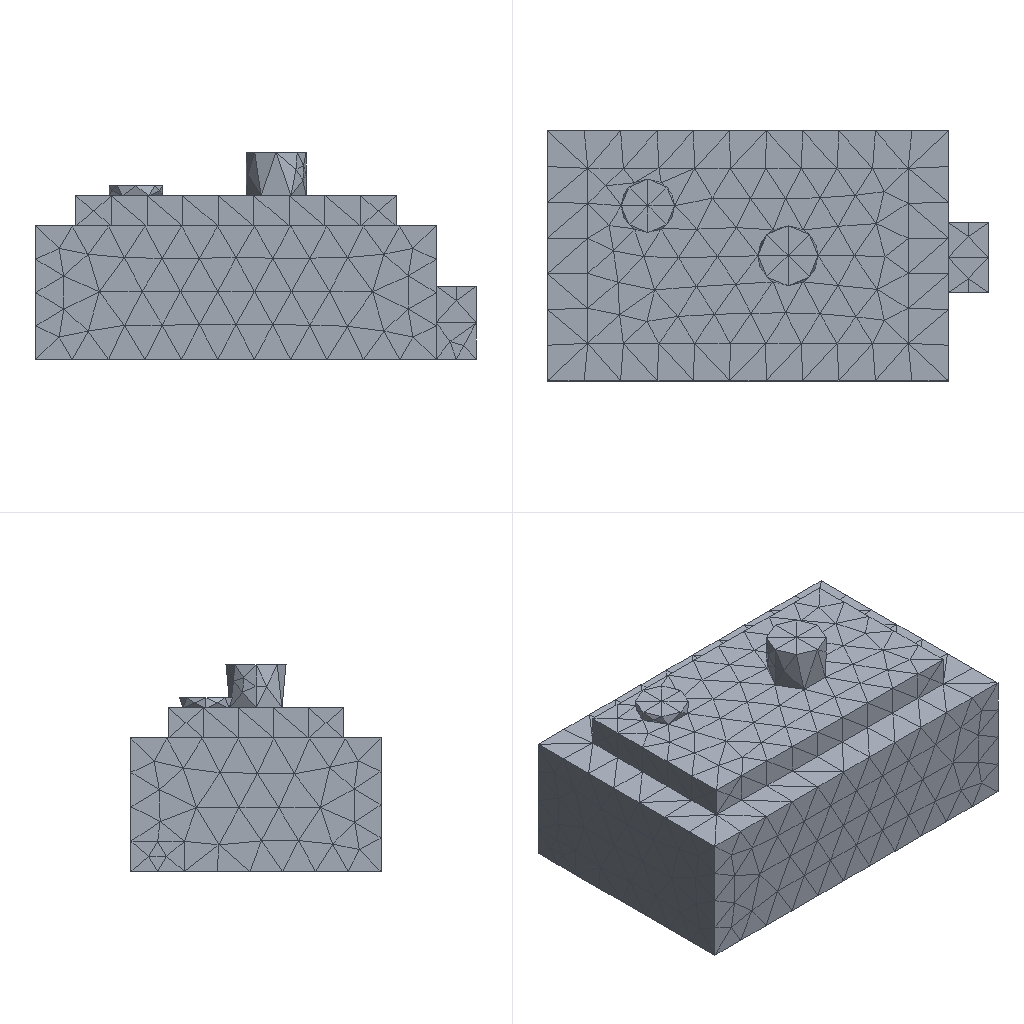Simulation study | ansys mapdl
Set-up summary:
category,name,step,type,value,unit,region
solver,ansys_mapdl
units,mm-N-s-tonne (MPa),,inferred,E=210000 density=
analysis,model,,static
mesh,nodes,,,4843
mesh,elements,,,2901
element_type,SOLID187,,,2901
material,mat 1,,E,210000
material,mat 1,,nu,0.3
load,,model,body load temp,,,all
load,,model,force,"1000 [dir=(0, 0, -1) n=211]",,node list
bc,,model,fixed,"[dofs=UX,UY,UZ n=5226]",,node list
Ansys APDL input file, long lists of numbers shortened:
/COM,ANSYS RELEASE 2026 R1           BUILD 26.1      UP20260202       09:08:46
/PREP7
/NOPR
/TITLE,2
ANTYPE, 0
*IF,_CDRDOFF,EQ,1,THEN     !if solid model was read in
_CDRDOFF=             !reset flag, numoffs already performed
*ELSE              !offset database for the following FE model
NUMOFF,NODE,     4843
NUMOFF,ELEM,     2901
NUMOFF,MAT ,        1
NUMOFF,TYPE,        1
*ENDIF
*SET,_RETURN ,  0.
*SET,_STATUS ,  0.
*SET,_UIQR   ,  211.
*SET,__FLOATPARAMETER__,  4843.
DOF,DELETE
ETBLOCK,        1,        1
(2i9,19a9)
        1      187        0        0        0        0        0        0        0        0        0        0        0        0        0        0        0        0        0        0        0
       -1
NBLOCK,6,SOLID,      4843,      4843
(3i9,6e21.13e3)
        1        0        0-4.4050000000000E+001 3.7500000000000E+001 9.0000000000000E+000
! (4842 more lines like these left out)
N,UNBL,LOC,       -1,
EBLOCK,19,SOLID,      2901,      2901
(19i10)
         1         1         1         1         0         0         0         0        10         0         1      1847      1570      1848      1569      2125      2126      2127      2128
! (5801 more lines like these left out)
        -1
MPTEMP,UNBL, 1, 1,  0.    ,
MPDATA,UNBL, 1,EX  ,       1, 1,  210000.000    ,
MPTEMP,UNBL, 1, 1,  0.    ,
MPDATA,UNBL, 1,NUXY,       1, 1, 0.3    ,
MPTEMP,UNBL, 1, 1,  0.    ,
MPDATA,UNBL, 1,PRXY,       1, 1, 0.3    ,
EXTOPT,ATTR,      0,      0,      0
EXTOPT,ESIZE,  0,  0.
EXTOPT,ACLEAR,      0
TREF,  0.
IRLF,  0
BFUNIF,TEMP,_TINY
ACEL,  0.    ,  0.    ,  0.
OMEGA,  0.    ,  0.    ,  0.
DOMEGA,  0.    ,  0.    ,  0.
CGLOC,  0.    ,  0.    ,  0.
CGOMEGA,  0.    ,  0.    ,  0.
DCGOMG,  0.    ,  0.    ,  0.
KUSE,     0
TIME,  0.
ALPHAD,  0.
BETAD,  0.
DMPRAT,  0.
DMPSTR,  0.
CRPLIM, 0.1    ,   0
CRPLIM,  0.    ,   1
NCNV,     0, 1.000000000E+12,     0,  0.    ,  0.
NEQIT,     0
ERESX,DEFA
DBLOCK,      5226
(i9,a6,2(pg16.9))
        1  UX    0.00000000      0.00000000
! (5225 more lines like these left out)
       -1
FBLOCK,       211
(i9,a6,2(pg16.9))
      884  FZ   -4.73933649      0.00000000
! (210 more lines like these left out)
       -1
/GO
FINISH
Results summary:
result,analysis_type_db,,,static,unstated
result,n_sets,,,1,unstated
result,load_steps[0].set,load_step=1,,1,unstated
result,load_steps[0].substep,load_step=1,,1,unstated
result,load_steps[0].time,load_step=1,,1,unstated
result,load_steps[0].freq,load_step=1,,1,unstated
result,load_steps[0].max_usum,load_step=1,,0.0003228,unstated
result,load_steps[0].max_seqv,load_step=1,,3.832,unstated
result,load_steps[0].reaction_sum.FX,load_step=1,,-4.44089e-12,unstated
result,load_steps[0].reaction_sum.FY,load_step=1,,-2.27374e-12,unstated
result,load_steps[0].reaction_sum.FZ,load_step=1,,1000,unstated
result,load_steps[0].reaction_sum.MX,load_step=1,,0,unstated
result,load_steps[0].reaction_sum.MY,load_step=1,,0,unstated
result,load_steps[0].reaction_sum.MZ,load_step=1,,0,unstated
result,convergence,,,results present for all listed sets,unstated